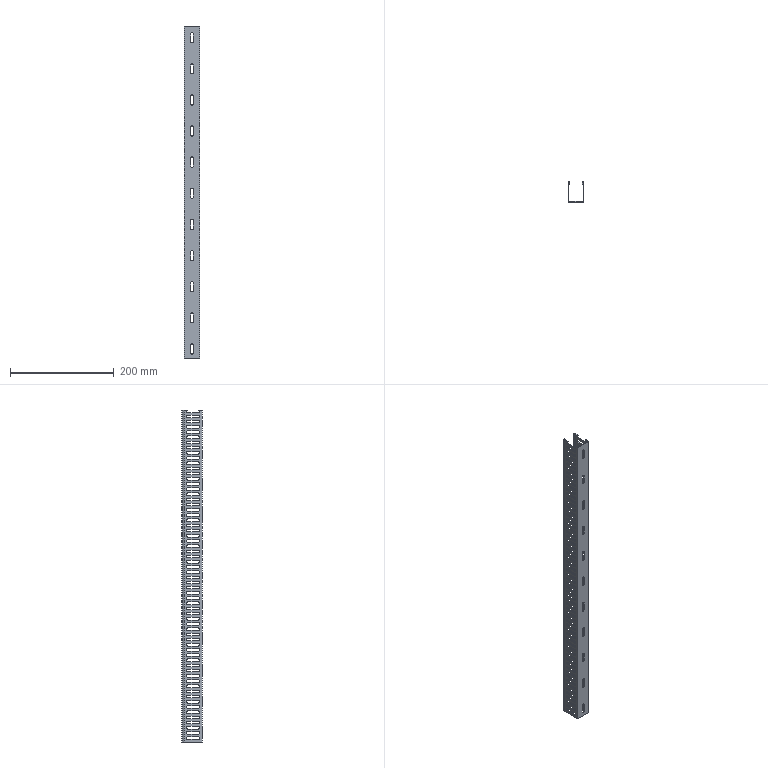Part | SolidWorks | features ICE 2, LPattern 2, Extrusion 1 | 1 solid | 728 faces | box 30 x 40 x 640 mm | volume 83874 mm3 | cylinder 430 | plane 298 | commonest cylinder face diameters 5 x417 1 x13